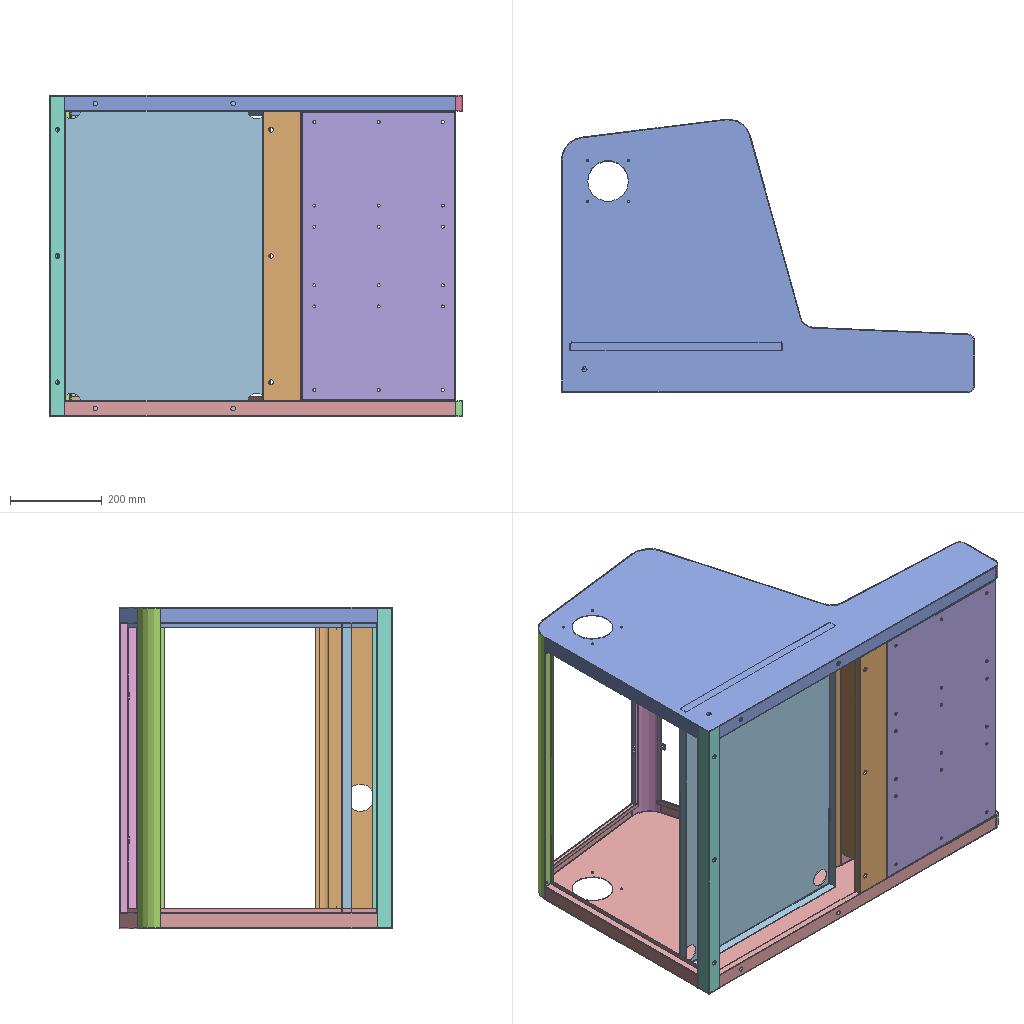Assembly | SolidWorks | 11 different items | 11 placed | box 900 x 595 x 700 mm
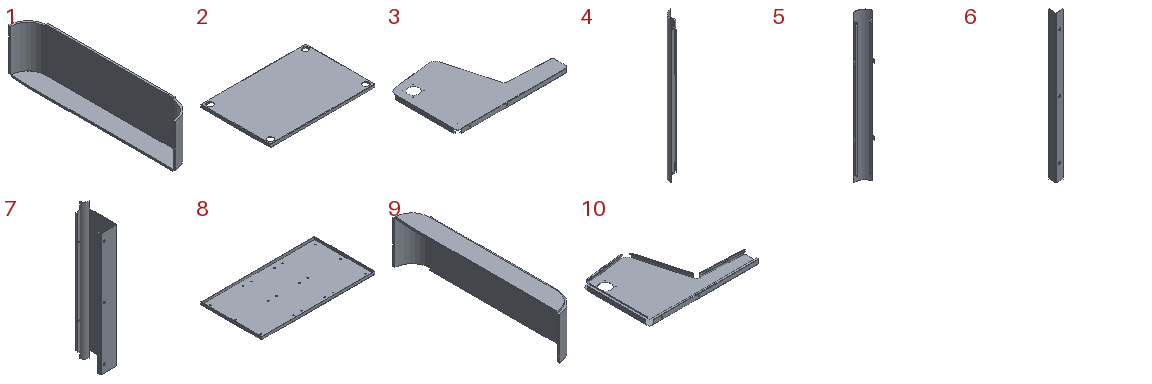Parts list (item | name | quantity | size | volume | features):
1 | - | x1 | 15 x 126.848 x 35 mm | 9537 mm3 | features SMBaseFlange 2, EdgeFlange 1, FlatPattern 1, ICE 1, SheetMetal 1
2 | - | x1 | 697 x 463 x 20 mm | 716512 mm3 | features Extrusion 1, FlatPattern 1, FlattenBends 1, ICE 1, ProcessBends 1, Rip 1, SheetMetal 1, Shell 1
3 | - | x1 | 898.5 x 594.649 x 48.5 mm | 675407 mm3 | features EdgeFlange 15, ICE 4, FlatPattern 1, SMBaseFlange 1, SheetMetal 1
4 | - | x1 | 56.016 x 59.625 x 700 mm | 123971 mm3 | features EdgeFlange 4, ICE 2, FlatPattern 1, SMBaseFlange 1, SheetMetal 1
5 | - | x1 | 72.164 x 60.825 x 700 mm | 123678 mm3 | features EdgeFlange 4, SMBaseFlange 3, ICE 2, FlatPattern 1, SheetMetal 1
6 | - | x1 | 35 x 43.5 x 700 mm | 106566 mm3 | features EdgeFlange 3, ICE 2, FlatPattern 1, LPattern 1, SMBaseFlange 1, SheetMetal 1
7 | - | x1 | 84 x 168.236 x 700 mm | 282210 mm3 | features EdgeFlange 4, ICE 4, FlatPattern 1, SMBaseFlange 1, SheetMetal 1
8 | - | x1 | 630 x 336 x 15 mm | 354650 mm3 | features Extrusion 1, FlatPattern 1, FlattenBends 1, ICE 1, ProcessBends 1, Rip 1, SheetMetal 1, Shell 1
9 | - | x1 | 15 x 126.848 x 35 mm | 9537 mm3 | features SMBaseFlange 2, EdgeFlange 1, FlatPattern 1, ICE 1, SheetMetal 1
10 | - | x1 | 898.5 x 594.649 x 48.5 mm | 675407 mm3 | features EdgeFlange 15, ICE 4, FlatPattern 1, SMBaseFlange 1, SheetMetal 1
11 | hexagon fit bolts--product grade a and b gb | x1 | - | - | -
Mates (type | each side: item.copy, entity, surface, feature):
Coincident | 3.1 face plane Base-Flange1 | 10.1 face plane Base-Flange1
DistanceDim | 3.1 face plane Base-Flange1 | 10.1 face plane Base-Flange1
Coincident | 10.1 face plane Edge-Flange5 | 3.1 face plane Edge-Flange5
Concentric | 3.1 face cylinder Base-Flange1 | 4.1 face cylinder Base-Flange1
Coincident | 3.1 face plane Base-Flange1 | 4.1 face plane Base-Flange1
Coincident | 3.1 face plane Edge-Flange1 | 4.1 face plane Base-Flange1
Concentric | 3.1 face cylinder Base-Flange1 | 5.1 face cylinder Base-Flange1
Coincident | 3.1 face plane Base-Flange1 | 5.1 face plane Base-Flange1
Coincident | 3.1 face plane Edge-Flange2 | 5.1 face plane Base-Flange1
Coincident | 3.1 face plane Base-Flange1 | 6.1 face plane Base-Flange1
Coincident | 3.1 face plane Edge-Flange5 | 6.1 face plane Base-Flange1
Coincident | 3.1 face plane Edge-Flange6 | 6.1 face plane Base-Flange1
Concentric | 3.1 face cylinder Base-Flange1 | 7.1 face cylinder Base-Flange2
Coincident | 3.1 face plane Base-Flange1 | 7.1 face plane Base-Flange2
Coincident | 3.1 face plane Edge-Flange2 | 7.1 face plane Base-Flange1
Coincident | 3.1 face plane Edge-Flange10 | 8.1 face plane Boss-Extrude1
Coincident | 3.1 face plane Edge-Flange5 | 8.1 face plane Boss-Extrude1
DistanceDim | 8.1 face plane Boss-Extrude1 | 3.1 face plane Base-Flange1
Coincident | 10.1 face plane Base-Flange1 | 9.1 face plane Base-Flange1 | 2 times
Concentric | 10.1 face cylinder Base-Flange1 | 9.1 face cylinder Base-Flange2
Coincident | 3.1 face plane Base-Flange1 | 1.1 face plane Base-Flange1 | 2 times
Concentric | 3.1 face cylinder Base-Flange1 | 1.1 face cylinder Base-Flange2
Coincident | 10.1 face plane Base-Flange1 | 2.1 face plane Boss-Extrude1
Coincident | 10.1 face plane Edge-Flange13 | 2.1 face plane Boss-Extrude1
DistanceDim | 2.1 face plane Boss-Extrude1 | 6.1 face plane Base-Flange1